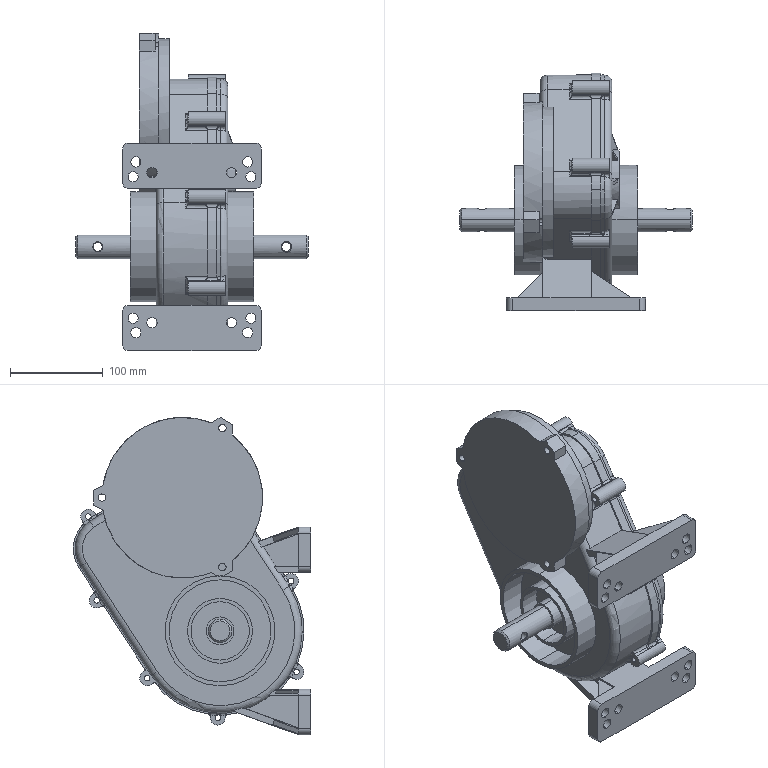Part | SolidWorks | features BaseBody 1 | 1 solid | 433 faces | box 251 x 256.191 x 342.363 mm | volume 4473281 mm3 | cylinder 223 | plane 154 | spline 31 | torus 21 | cone 4 | commonest cylinder face diameters 6 x113 11 x24 16 x12 13.2 x8 63 x7 177 x7